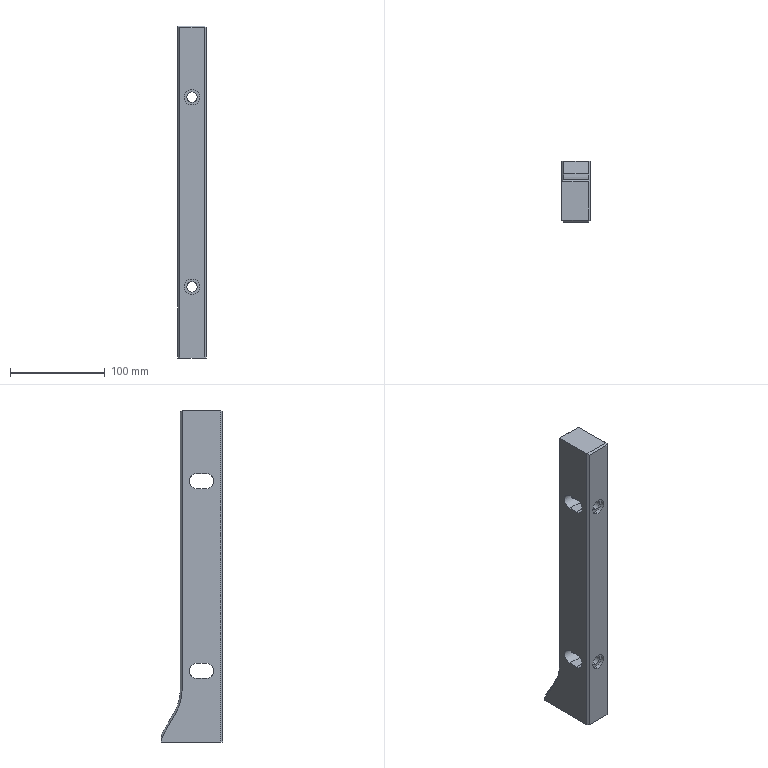Part | STEP file | Screen clamp fixing plate^Right screen clamp assembly_Screen assembly_PS-3045E-LDJ2 | 1 solid | 60 faces | box 30 x 64.5 x 350 mm | volume 452377 mm3 | cylinder 25 | plane 25 | cone 10 | commonest cylinder face diameters 5 x8 11 x8 16 x4 16.5 x4 100 x1